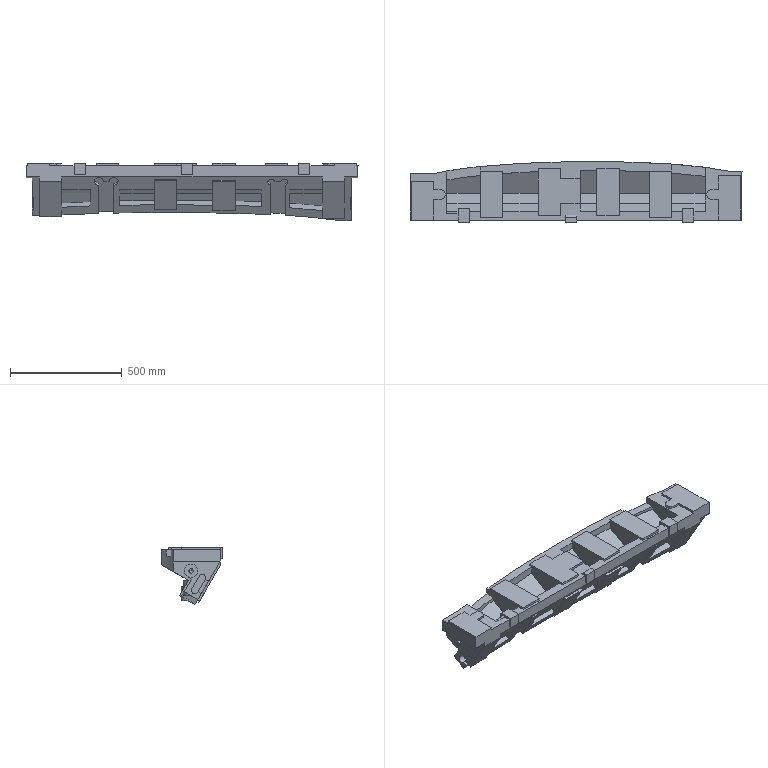Part | NX | features MAIN_BODY 2 | 1 solid | 270 faces | box 1487 x 272.345 x 255.84 mm | volume 40715146 mm3 | plane 228 | cylinder 26 | spline 12 | cone 4 | commonest cylinder face diameters 60 x9 20 x7 32 x6 40 x2 45 x2